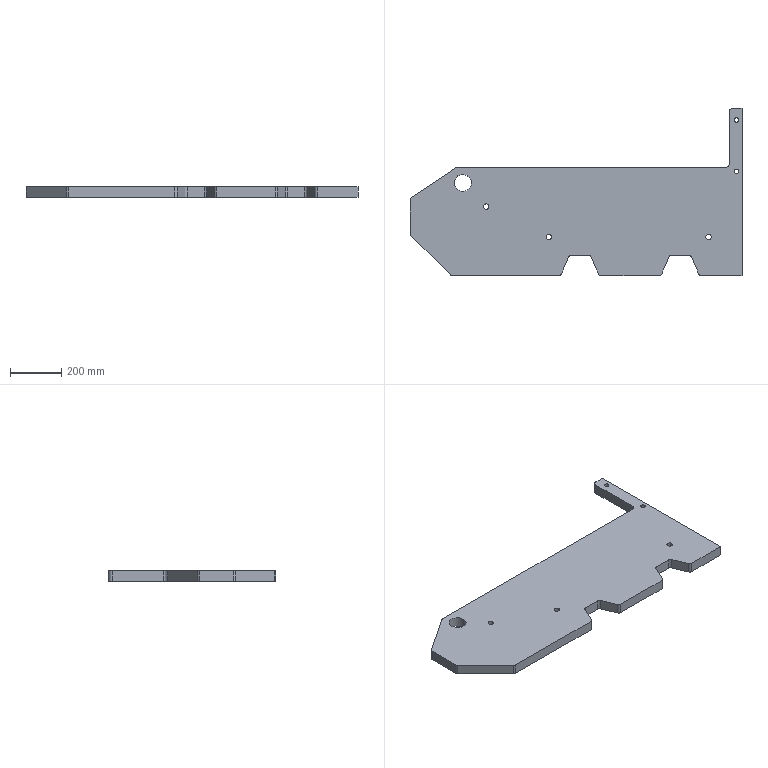Part | SolidWorks | features Fillet 3, Chamfer 2, 3DProfileFeature 1, Extrusion 1, HoleWzd 1, ICE 1 | 1 solid | 44 faces | box 1290 x 650 x 40 mm | volume 20252849 mm3 | cylinder 26 | plane 18 | commonest cylinder face diameters 20 x12 21 x6 18 x4 30 x2 66 x2
STEP:
#1=CARTESIAN_POINT('',(550.5,150.,0.));
#2=VERTEX_POINT('',#1);
#3=CARTESIAN_POINT('',(529.5,150.,0.));
#4=VERTEX_POINT('',#3);
#5=CARTESIAN_POINT('',(540.,150.,0.));
#6=DIRECTION('',(0.,0.,-1.));
#7=DIRECTION('',(-1.,0.,0.));
#8=AXIS2_PLACEMENT_3D('',#5,#6,#7);
#9=CIRCLE('',#8,10.5);
#10=EDGE_CURVE('',#2,#4,#9,.T.);
#11=ORIENTED_EDGE('',*,*,#10,.T.);
#12=CARTESIAN_POINT('',(529.5,150.,40.));
#13=VERTEX_POINT('',#12);
#14=CARTESIAN_POINT('',(529.5,150.,40.));
#15=DIRECTION('',(0.,0.,1.));
#16=VECTOR('',#15,1000.);
#17=LINE('',#14,#16);
#18=EDGE_CURVE('',#4,#13,#17,.T.);
#19=ORIENTED_EDGE('',*,*,#18,.T.);
#20=CARTESIAN_POINT('',(550.5,150.,40.));
#21=VERTEX_POINT('',#20);
#22=CARTESIAN_POINT('',(540.,150.,40.));
#23=DIRECTION('',(0.,0.,1.));
#24=DIRECTION('',(1.,0.,0.));
#25=AXIS2_PLACEMENT_3D('',#22,#23,#24);
#26=CIRCLE('',#25,10.5);
#27=EDGE_CURVE('',#13,#21,#26,.T.);
#28=ORIENTED_EDGE('',*,*,#27,.T.);
#29=CARTESIAN_POINT('',(550.5,150.,40.));
#30=DIRECTION('',(0.,0.,1.));
#31=VECTOR('',#30,1000.);
#32=LINE('',#29,#31);
#33=EDGE_CURVE('',#2,#21,#32,.T.);
#34=ORIENTED_EDGE('',*,*,#33,.F.);
#35=EDGE_LOOP('',(#11,#19,#28,#34));
#36=FACE_OUTER_BOUND('',#35,.T.);
#37=CARTESIAN_POINT('',(540.,150.,40.));
#38=DIRECTION('',(0.,0.,1.));
#39=DIRECTION('',(1.,0.,0.));
#40=AXIS2_PLACEMENT_3D('',#37,#38,#39);
#41=CYLINDRICAL_SURFACE('',#40,10.5);
#42=ADVANCED_FACE('',(#36),#41,.F.);
#43=CARTESIAN_POINT('',(1170.5,150.,0.));
#44=VERTEX_POINT('',#43);
#45=CARTESIAN_POINT('',(1149.5,150.,0.));
#46=VERTEX_POINT('',#45);
#47=CARTESIAN_POINT('',(1160.,150.,0.));
#48=DIRECTION('',(0.,0.,-1.));
#49=DIRECTION('',(-1.,0.,0.));
#50=AXIS2_PLACEMENT_3D('',#47,#48,#49);
#51=CIRCLE('',#50,10.5);
#52=EDGE_CURVE('',#44,#46,#51,.T.);
#53=ORIENTED_EDGE('',*,*,#52,.T.);
#54=CARTESIAN_POINT('',(1149.5,150.,40.));
#55=VERTEX_POINT('',#54);
#56=CARTESIAN_POINT('',(1149.5,150.,40.));
#57=DIRECTION('',(0.,0.,1.));
#58=VECTOR('',#57,1000.);
#59=LINE('',#56,#58);
#60=EDGE_CURVE('',#46,#55,#59,.T.);
#61=ORIENTED_EDGE('',*,*,#60,.T.);
#62=CARTESIAN_POINT('',(1170.5,150.,40.));
#63=VERTEX_POINT('',#62);
#64=CARTESIAN_POINT('',(1160.,150.,40.));
#65=DIRECTION('',(0.,0.,1.));
#66=DIRECTION('',(1.,0.,0.));
#67=AXIS2_PLACEMENT_3D('',#64,#65,#66);
#68=CIRCLE('',#67,10.5);
#69=EDGE_CURVE('',#55,#63,#68,.T.);
#70=ORIENTED_EDGE('',*,*,#69,.T.);
#71=CARTESIAN_POINT('',(1170.5,150.,40.));
#72=DIRECTION('',(0.,0.,1.));
#73=VECTOR('',#72,1000.);
#74=LINE('',#71,#73);
#75=EDGE_CURVE('',#44,#63,#74,.T.);
#76=ORIENTED_EDGE('',*,*,#75,.F.);
#77=EDGE_LOOP('',(#53,#61,#70,#76));
#78=FACE_OUTER_BOUND('',#77,.T.);
#79=CARTESIAN_POINT('',(1160.,150.,40.));
#80=DIRECTION('',(0.,0.,1.));
#81=DIRECTION('',(1.,0.,0.));
#82=AXIS2_PLACEMENT_3D('',#79,#80,#81);
#83=CYLINDRICAL_SURFACE('',#82,10.5);
#84=ADVANCED_FACE('',(#78),#83,.F.);
#85=CARTESIAN_POINT('',(306.435,268.316,0.));
#86=VERTEX_POINT('',#85);
#87=CARTESIAN_POINT('',(285.435,268.316,0.));
#88=VERTEX_POINT('',#87);
#89=CARTESIAN_POINT('',(295.935,268.316,0.));
#90=DIRECTION('',(0.,0.,-1.));
#91=DIRECTION('',(-1.,0.,0.));
#92=AXIS2_PLACEMENT_3D('',#89,#90,#91);
#93=CIRCLE('',#92,10.5);
#94=EDGE_CURVE('',#86,#88,#93,.T.);
#95=ORIENTED_EDGE('',*,*,#94,.T.);
#96=CARTESIAN_POINT('',(285.435,268.316,40.));
#97=VERTEX_POINT('',#96);
#98=CARTESIAN_POINT('',(285.435,268.316,40.));
#99=DIRECTION('',(0.,0.,1.));
#100=VECTOR('',#99,1000.);
#101=LINE('',#98,#100);
#102=EDGE_CURVE('',#88,#97,#101,.T.);
#103=ORIENTED_EDGE('',*,*,#102,.T.);
#104=CARTESIAN_POINT('',(306.435,268.316,40.));
#105=VERTEX_POINT('',#104);
#106=CARTESIAN_POINT('',(295.935,268.316,40.));
#107=DIRECTION('',(0.,0.,1.));
#108=DIRECTION('',(1.,0.,0.));
#109=AXIS2_PLACEMENT_3D('',#106,#107,#108);
#110=CIRCLE('',#109,10.5);
#111=EDGE_CURVE('',#97,#105,#110,.T.);
#112=ORIENTED_EDGE('',*,*,#111,.T.);
#113=CARTESIAN_POINT('',(306.435,268.316,40.));
#114=DIRECTION('',(0.,0.,1.));
#115=VECTOR('',#114,1000.);
#116=LINE('',#113,#115);
#117=EDGE_CURVE('',#86,#105,#116,.T.);
#118=ORIENTED_EDGE('',*,*,#117,.F.);
#119=EDGE_LOOP('',(#95,#103,#112,#118));
#120=FACE_OUTER_BOUND('',#119,.T.);
#121=CARTESIAN_POINT('',(295.935,268.316,40.));
#122=DIRECTION('',(0.,0.,1.));
#123=DIRECTION('',(1.,0.,0.));
#124=AXIS2_PLACEMENT_3D('',#121,#122,#123);
#125=CYLINDRICAL_SURFACE('',#124,10.5);
#126=ADVANCED_FACE('',(#120),#125,.F.);
#127=CARTESIAN_POINT('',(1260.,405.,40.));
#128=VERTEX_POINT('',#127);
#129=CARTESIAN_POINT('',(1278.,405.,40.));
#130=VERTEX_POINT('',#129);
#131=CARTESIAN_POINT('',(1269.,405.,40.));
#132=DIRECTION('',(0.,0.,1.));
#133=DIRECTION('',(1.,0.,0.));
#134=AXIS2_PLACEMENT_3D('',#131,#132,#133);
#135=CIRCLE('',#134,9.);
#136=EDGE_CURVE('',#128,#130,#135,.T.);
#137=ORIENTED_EDGE('',*,*,#136,.T.);
#138=CARTESIAN_POINT('',(1278.,405.,0.));
#139=VERTEX_POINT('',#138);
#140=CARTESIAN_POINT('',(1278.,405.,40.));
#141=DIRECTION('',(0.,0.,-1.));
#142=VECTOR('',#141,1000.);
#143=LINE('',#140,#142);
#144=EDGE_CURVE('',#130,#139,#143,.T.);
#145=ORIENTED_EDGE('',*,*,#144,.T.);
#146=CARTESIAN_POINT('',(1260.,405.,0.));
#147=VERTEX_POINT('',#146);
#148=CARTESIAN_POINT('',(1269.,405.,0.));
#149=DIRECTION('',(0.,0.,1.));
#150=DIRECTION('',(1.,0.,0.));
#151=AXIS2_PLACEMENT_3D('',#148,#149,#150);
#152=CIRCLE('',#151,9.);
#153=EDGE_CURVE('',#147,#139,#152,.T.);
#154=ORIENTED_EDGE('',*,*,#153,.F.);
#155=CARTESIAN_POINT('',(1260.,405.,40.));
#156=DIRECTION('',(0.,0.,-1.));
#157=VECTOR('',#156,1000.);
#158=LINE('',#155,#157);
#159=EDGE_CURVE('',#128,#147,#158,.T.);
#160=ORIENTED_EDGE('',*,*,#159,.F.);
#161=EDGE_LOOP('',(#137,#145,#154,#160));
#162=FACE_OUTER_BOUND('',#161,.T.);
#163=CARTESIAN_POINT('',(1269.,405.,40.));
#164=DIRECTION('',(0.,0.,-1.));
#165=DIRECTION('',(-1.,0.,0.));
#166=AXIS2_PLACEMENT_3D('',#163,#164,#165);
#167=CYLINDRICAL_SURFACE('',#166,9.);
#168=ADVANCED_FACE('',(#162),#167,.F.);
#169=CARTESIAN_POINT('',(1260.,605.,40.));
#170=VERTEX_POINT('',#169);
#171=CARTESIAN_POINT('',(1278.,605.,40.));
#172=VERTEX_POINT('',#171);
#173=CARTESIAN_POINT('',(1269.,605.,40.));
#174=DIRECTION('',(0.,0.,1.));
#175=DIRECTION('',(1.,0.,0.));
#176=AXIS2_PLACEMENT_3D('',#173,#174,#175);
#177=CIRCLE('',#176,9.);
#178=EDGE_CURVE('',#170,#172,#177,.T.);
#179=ORIENTED_EDGE('',*,*,#178,.T.);
#180=CARTESIAN_POINT('',(1278.,605.,0.));
#181=VERTEX_POINT('',#180);
#182=CARTESIAN_POINT('',(1278.,605.,40.));
#183=DIRECTION('',(0.,0.,-1.));
#184=VECTOR('',#183,1000.);
#185=LINE('',#182,#184);
#186=EDGE_CURVE('',#172,#181,#185,.T.);
#187=ORIENTED_EDGE('',*,*,#186,.T.);
#188=CARTESIAN_POINT('',(1260.,605.,0.));
#189=VERTEX_POINT('',#188);
#190=CARTESIAN_POINT('',(1269.,605.,0.));
#191=DIRECTION('',(0.,0.,1.));
#192=DIRECTION('',(1.,0.,0.));
#193=AXIS2_PLACEMENT_3D('',#190,#191,#192);
#194=CIRCLE('',#193,9.);
#195=EDGE_CURVE('',#189,#181,#194,.T.);
#196=ORIENTED_EDGE('',*,*,#195,.F.);
#197=CARTESIAN_POINT('',(1260.,605.,40.));
#198=DIRECTION('',(0.,0.,-1.));
#199=VECTOR('',#198,1000.);
#200=LINE('',#197,#199);
#201=EDGE_CURVE('',#170,#189,#200,.T.);
#202=ORIENTED_EDGE('',*,*,#201,.F.);
#203=EDGE_LOOP('',(#179,#187,#196,#202));
#204=FACE_OUTER_BOUND('',#203,.T.);
#205=CARTESIAN_POINT('',(1269.,605.,40.));
#206=DIRECTION('',(0.,0.,-1.));
#207=DIRECTION('',(-1.,0.,0.));
#208=AXIS2_PLACEMENT_3D('',#205,#206,#207);
#209=CYLINDRICAL_SURFACE('',#208,9.);
#210=ADVANCED_FACE('',(#204),#209,.F.);
#211=CARTESIAN_POINT('',(172.,360.,40.));
#212=VERTEX_POINT('',#211);
#213=CARTESIAN_POINT('',(238.,360.,40.));
#214=VERTEX_POINT('',#213);
#215=CARTESIAN_POINT('',(205.,360.,40.));
#216=DIRECTION('',(0.,0.,1.));
#217=DIRECTION('',(1.,0.,0.));
#218=AXIS2_PLACEMENT_3D('',#215,#216,#217);
#219=CIRCLE('',#218,33.);
#220=EDGE_CURVE('',#212,#214,#219,.T.);
#221=ORIENTED_EDGE('',*,*,#220,.T.);
#222=CARTESIAN_POINT('',(238.,360.,0.));
#223=VERTEX_POINT('',#222);
#224=CARTESIAN_POINT('',(238.,360.,40.));
#225=DIRECTION('',(0.,0.,-1.));
#226=VECTOR('',#225,1000.);
#227=LINE('',#224,#226);
#228=EDGE_CURVE('',#214,#223,#227,.T.);
#229=ORIENTED_EDGE('',*,*,#228,.T.);
#230=CARTESIAN_POINT('',(172.,360.,0.));
#231=VERTEX_POINT('',#230);
#232=CARTESIAN_POINT('',(205.,360.,0.));
#233=DIRECTION('',(0.,0.,1.));
#234=DIRECTION('',(1.,0.,0.));
#235=AXIS2_PLACEMENT_3D('',#232,#233,#234);
#236=CIRCLE('',#235,33.);
#237=EDGE_CURVE('',#231,#223,#236,.T.);
#238=ORIENTED_EDGE('',*,*,#237,.F.);
#239=CARTESIAN_POINT('',(172.,360.,40.));
#240=DIRECTION('',(0.,0.,-1.));
#241=VECTOR('',#240,1000.);
#242=LINE('',#239,#241);
#243=EDGE_CURVE('',#212,#231,#242,.T.);
#244=ORIENTED_EDGE('',*,*,#243,.F.);
#245=EDGE_LOOP('',(#221,#229,#238,#244));
#246=FACE_OUTER_BOUND('',#245,.T.);
#247=CARTESIAN_POINT('',(205.,360.,40.));
#248=DIRECTION('',(0.,0.,-1.));
#249=DIRECTION('',(-1.,0.,0.));
#250=AXIS2_PLACEMENT_3D('',#247,#248,#249);
#251=CYLINDRICAL_SURFACE('',#250,33.);
#252=ADVANCED_FACE('',(#246),#251,.F.);
#253=CARTESIAN_POINT('',(1131.54,0.,40.));
#254=VERTEX_POINT('',#253);
#255=CARTESIAN_POINT('',(1290.,0.,40.));
#256=VERTEX_POINT('',#255);
#257=CARTESIAN_POINT('',(0.,0.,40.));
#258=DIRECTION('',(1.,0.,0.));
#259=VECTOR('',#258,1000.);
#260=LINE('',#257,#259);
#261=EDGE_CURVE('',#254,#256,#260,.T.);
#262=ORIENTED_EDGE('',*,*,#261,.F.);
#263=CARTESIAN_POINT('',(1131.54,0.,0.));
#264=VERTEX_POINT('',#263);
#265=CARTESIAN_POINT('',(1131.54,0.,40.));
#266=DIRECTION('',(0.,0.,-1.));
#267=VECTOR('',#266,1000.);
#268=LINE('',#265,#267);
#269=EDGE_CURVE('',#254,#264,#268,.T.);
#270=ORIENTED_EDGE('',*,*,#269,.T.);
#271=CARTESIAN_POINT('',(1290.,0.,0.));
#272=VERTEX_POINT('',#271);
#273=CARTESIAN_POINT('',(0.,0.,0.));
#274=DIRECTION('',(1.,0.,0.));
#275=VECTOR('',#274,1000.);
#276=LINE('',#273,#275);
#277=EDGE_CURVE('',#264,#272,#276,.T.);
#278=ORIENTED_EDGE('',*,*,#277,.T.);
#279=CARTESIAN_POINT('',(1290.,0.,40.));
#280=DIRECTION('',(0.,0.,-1.));
#281=VECTOR('',#280,1000.);
#282=LINE('',#279,#281);
#283=EDGE_CURVE('',#256,#272,#282,.T.);
#284=ORIENTED_EDGE('',*,*,#283,.F.);
#285=EDGE_LOOP('',(#262,#270,#278,#284));
#286=FACE_OUTER_BOUND('',#285,.T.);
#287=CARTESIAN_POINT('',(0.,0.,40.));
#288=DIRECTION('',(0.,1.,0.));
#289=DIRECTION('',(0.,0.,1.));
#290=AXIS2_PLACEMENT_3D('',#287,#288,#289);
#291=PLANE('',#290);
#292=ADVANCED_FACE('',(#286),#291,.F.);
#293=CARTESIAN_POINT('',(741.54,0.,0.));
#294=VERTEX_POINT('',#293);
#295=CARTESIAN_POINT('',(968.46,0.,0.));
#296=VERTEX_POINT('',#295);
#297=CARTESIAN_POINT('',(0.,0.,0.));
#298=DIRECTION('',(1.,0.,0.));
#299=VECTOR('',#298,1000.);
#300=LINE('',#297,#299);
#301=EDGE_CURVE('',#294,#296,#300,.T.);
#302=ORIENTED_EDGE('',*,*,#301,.T.);
#303=CARTESIAN_POINT('',(968.46,0.,40.));
#304=VERTEX_POINT('',#303);
#305=CARTESIAN_POINT('',(968.46,0.,40.));
#306=DIRECTION('',(0.,0.,1.));
#307=VECTOR('',#306,1000.);
#308=LINE('',#305,#307);
#309=EDGE_CURVE('',#296,#304,#308,.T.);
#310=ORIENTED_EDGE('',*,*,#309,.T.);
#311=CARTESIAN_POINT('',(741.54,0.,40.));
#312=VERTEX_POINT('',#311);
#313=CARTESIAN_POINT('',(0.,0.,40.));
#314=DIRECTION('',(1.,0.,0.));
#315=VECTOR('',#314,1000.);
#316=LINE('',#313,#315);
#317=EDGE_CURVE('',#312,#304,#316,.T.);
#318=ORIENTED_EDGE('',*,*,#317,.F.);
#319=CARTESIAN_POINT('',(741.54,0.,40.));
#320=DIRECTION('',(0.,0.,-1.));
#321=VECTOR('',#320,1000.);
#322=LINE('',#319,#321);
#323=EDGE_CURVE('',#312,#294,#322,.T.);
#324=ORIENTED_EDGE('',*,*,#323,.T.);
#325=EDGE_LOOP('',(#302,#310,#318,#324));
#326=FACE_OUTER_BOUND('',#325,.T.);
#327=CARTESIAN_POINT('',(0.,0.,40.));
#328=DIRECTION('',(0.,1.,0.));
#329=DIRECTION('',(0.,0.,1.));
#330=AXIS2_PLACEMENT_3D('',#327,#328,#329);
#331=PLANE('',#330);
#332=ADVANCED_FACE('',(#326),#331,.F.);
#333=CARTESIAN_POINT('',(540.,150.,40.));
#334=DIRECTION('',(0.,0.,1.));
#335=DIRECTION('',(1.,0.,0.));
#336=AXIS2_PLACEMENT_3D('',#333,#334,#335);
#337=CIRCLE('',#336,10.5);
#338=EDGE_CURVE('',#21,#13,#337,.T.);
#339=ORIENTED_EDGE('',*,*,#338,.F.);
#340=ORIENTED_EDGE('',*,*,#27,.F.);
#341=EDGE_LOOP('',(#339,#340));
#342=FACE_BOUND('',#341,.T.);
#343=CARTESIAN_POINT('',(2.929,157.071,40.));
#344=VERTEX_POINT('',#343);
#345=CARTESIAN_POINT('',(157.071,2.929,40.));
#346=VERTEX_POINT('',#345);
#347=CARTESIAN_POINT('',(160.,0.,40.));
#348=DIRECTION('',(0.7071,-0.7071,0.));
#349=VECTOR('',#348,1000.);
#350=LINE('',#347,#349);
#351=EDGE_CURVE('',#344,#346,#350,.T.);
#352=ORIENTED_EDGE('',*,*,#351,.T.);
#353=CARTESIAN_POINT('',(164.142,0.,40.));
#354=VERTEX_POINT('',#353);
#355=CARTESIAN_POINT('',(164.142,10.,40.));
#356=DIRECTION('',(0.,0.,1.));
#357=DIRECTION('',(-1.,0.,0.));
#358=AXIS2_PLACEMENT_3D('',#355,#356,#357);
#359=CIRCLE('',#358,10.);
#360=EDGE_CURVE('',#346,#354,#359,.T.);
#361=ORIENTED_EDGE('',*,*,#360,.T.);
#362=CARTESIAN_POINT('',(578.46,0.,40.));
#363=VERTEX_POINT('',#362);
#364=CARTESIAN_POINT('',(0.,0.,40.));
#365=DIRECTION('',(1.,0.,0.));
#366=VECTOR('',#365,1000.);
#367=LINE('',#364,#366);
#368=EDGE_CURVE('',#354,#363,#367,.T.);
#369=ORIENTED_EDGE('',*,*,#368,.T.);
#370=CARTESIAN_POINT('',(587.621,5.992,40.));
#371=VERTEX_POINT('',#370);
#372=CARTESIAN_POINT('',(578.46,10.,40.));
#373=DIRECTION('',(0.,0.,1.));
#374=DIRECTION('',(-1.,0.,0.));
#375=AXIS2_PLACEMENT_3D('',#372,#373,#374);
#376=CIRCLE('',#375,10.);
#377=EDGE_CURVE('',#363,#371,#376,.T.);
#378=ORIENTED_EDGE('',*,*,#377,.T.);
#379=CARTESIAN_POINT('',(617.379,74.008,40.));
#380=VERTEX_POINT('',#379);
#381=CARTESIAN_POINT('',(620.,80.,40.));
#382=DIRECTION('',(-0.4008,-0.9162,0.));
#383=VECTOR('',#382,1000.);
#384=LINE('',#381,#383);
#385=EDGE_CURVE('',#380,#371,#384,.T.);
#386=ORIENTED_EDGE('',*,*,#385,.F.);
#387=CARTESIAN_POINT('',(626.54,80.,40.));
#388=VERTEX_POINT('',#387);
#389=CARTESIAN_POINT('',(626.54,70.,40.));
#390=DIRECTION('',(0.,0.,-1.));
#391=DIRECTION('',(-1.,0.,0.));
#392=AXIS2_PLACEMENT_3D('',#389,#390,#391);
#393=CIRCLE('',#392,10.);
#394=EDGE_CURVE('',#380,#388,#393,.T.);
#395=ORIENTED_EDGE('',*,*,#394,.T.);
#396=CARTESIAN_POINT('',(693.46,80.,40.));
#397=VERTEX_POINT('',#396);
#398=CARTESIAN_POINT('',(620.,80.,40.));
#399=DIRECTION('',(-1.,0.,0.));
#400=VECTOR('',#399,1000.);
#401=LINE('',#398,#400);
#402=EDGE_CURVE('',#397,#388,#401,.T.);
#403=ORIENTED_EDGE('',*,*,#402,.F.);
#404=CARTESIAN_POINT('',(702.621,74.008,40.));
#405=VERTEX_POINT('',#404);
#406=CARTESIAN_POINT('',(693.46,70.,40.));
#407=DIRECTION('',(0.,0.,-1.));
#408=DIRECTION('',(-1.,0.,0.));
#409=AXIS2_PLACEMENT_3D('',#406,#407,#408);
#410=CIRCLE('',#409,10.);
#411=EDGE_CURVE('',#397,#405,#410,.T.);
#412=ORIENTED_EDGE('',*,*,#411,.T.);
#413=CARTESIAN_POINT('',(732.379,5.992,40.));
#414=VERTEX_POINT('',#413);
#415=CARTESIAN_POINT('',(700.,80.,40.));
#416=DIRECTION('',(-0.4008,0.9162,0.));
#417=VECTOR('',#416,1000.);
#418=LINE('',#415,#417);
#419=EDGE_CURVE('',#414,#405,#418,.T.);
#420=ORIENTED_EDGE('',*,*,#419,.F.);
#421=CARTESIAN_POINT('',(741.54,10.,40.));
#422=DIRECTION('',(0.,0.,1.));
#423=DIRECTION('',(-1.,0.,0.));
#424=AXIS2_PLACEMENT_3D('',#421,#422,#423);
#425=CIRCLE('',#424,10.);
#426=EDGE_CURVE('',#414,#312,#425,.T.);
#427=ORIENTED_EDGE('',*,*,#426,.T.);
#428=ORIENTED_EDGE('',*,*,#317,.T.);
#429=CARTESIAN_POINT('',(977.621,5.992,40.));
#430=VERTEX_POINT('',#429);
#431=CARTESIAN_POINT('',(968.46,10.,40.));
#432=DIRECTION('',(0.,0.,1.));
#433=DIRECTION('',(-1.,0.,0.));
#434=AXIS2_PLACEMENT_3D('',#431,#432,#433);
#435=CIRCLE('',#434,10.);
#436=EDGE_CURVE('',#304,#430,#435,.T.);
#437=ORIENTED_EDGE('',*,*,#436,.T.);
#438=CARTESIAN_POINT('',(1007.379,74.008,40.));
#439=VERTEX_POINT('',#438);
#440=CARTESIAN_POINT('',(1010.,80.,40.));
#441=DIRECTION('',(-0.4008,-0.9162,0.));
#442=VECTOR('',#441,1000.);
#443=LINE('',#440,#442);
#444=EDGE_CURVE('',#439,#430,#443,.T.);
#445=ORIENTED_EDGE('',*,*,#444,.F.);
#446=CARTESIAN_POINT('',(1016.54,80.,40.));
#447=VERTEX_POINT('',#446);
#448=CARTESIAN_POINT('',(1016.54,70.,40.));
#449=DIRECTION('',(0.,0.,-1.));
#450=DIRECTION('',(-1.,0.,0.));
#451=AXIS2_PLACEMENT_3D('',#448,#449,#450);
#452=CIRCLE('',#451,10.);
#453=EDGE_CURVE('',#439,#447,#452,.T.);
#454=ORIENTED_EDGE('',*,*,#453,.T.);
#455=CARTESIAN_POINT('',(1083.46,80.,40.));
#456=VERTEX_POINT('',#455);
#457=CARTESIAN_POINT('',(1010.,80.,40.));
#458=DIRECTION('',(-1.,0.,0.));
#459=VECTOR('',#458,1000.);
#460=LINE('',#457,#459);
#461=EDGE_CURVE('',#456,#447,#460,.T.);
#462=ORIENTED_EDGE('',*,*,#461,.F.);
#463=CARTESIAN_POINT('',(1092.621,74.008,40.));
#464=VERTEX_POINT('',#463);
#465=CARTESIAN_POINT('',(1083.46,70.,40.));
#466=DIRECTION('',(0.,0.,-1.));
#467=DIRECTION('',(-1.,0.,0.));
#468=AXIS2_PLACEMENT_3D('',#465,#466,#467);
#469=CIRCLE('',#468,10.);
#470=EDGE_CURVE('',#456,#464,#469,.T.);
#471=ORIENTED_EDGE('',*,*,#470,.T.);
#472=CARTESIAN_POINT('',(1122.379,5.992,40.));
#473=VERTEX_POINT('',#472);
#474=CARTESIAN_POINT('',(1090.,80.,40.));
#475=DIRECTION('',(-0.4008,0.9162,0.));
#476=VECTOR('',#475,1000.);
#477=LINE('',#474,#476);
#478=EDGE_CURVE('',#473,#464,#477,.T.);
#479=ORIENTED_EDGE('',*,*,#478,.F.);
#480=CARTESIAN_POINT('',(1131.54,10.,40.));
#481=DIRECTION('',(0.,0.,1.));
#482=DIRECTION('',(-1.,0.,0.));
#483=AXIS2_PLACEMENT_3D('',#480,#481,#482);
#484=CIRCLE('',#483,10.);
#485=EDGE_CURVE('',#473,#254,#484,.T.);
#486=ORIENTED_EDGE('',*,*,#485,.T.);
#487=ORIENTED_EDGE('',*,*,#261,.T.);
#488=CARTESIAN_POINT('',(1290.,650.,40.));
#489=VERTEX_POINT('',#488);
#490=CARTESIAN_POINT('',(1290.,0.,40.));
#491=DIRECTION('',(0.,1.,0.));
#492=VECTOR('',#491,1000.);
#493=LINE('',#490,#492);
#494=EDGE_CURVE('',#256,#489,#493,.T.);
#495=ORIENTED_EDGE('',*,*,#494,.T.);
#496=CARTESIAN_POINT('',(1255.,650.,40.));
#497=VERTEX_POINT('',#496);
#498=CARTESIAN_POINT('',(1240.,650.,40.));
#499=DIRECTION('',(-1.,0.,0.));
#500=VECTOR('',#499,1000.);
#501=LINE('',#498,#500);
#502=EDGE_CURVE('',#489,#497,#501,.T.);
#503=ORIENTED_EDGE('',*,*,#502,.T.);
#504=CARTESIAN_POINT('',(1240.,635.,40.));
#505=VERTEX_POINT('',#504);
#506=CARTESIAN_POINT('',(1255.,635.,40.));
#507=DIRECTION('',(0.,0.,1.));
#508=DIRECTION('',(-1.,0.,0.));
#509=AXIS2_PLACEMENT_3D('',#506,#507,#508);
#510=CIRCLE('',#509,15.);
#511=EDGE_CURVE('',#497,#505,#510,.T.);
#512=ORIENTED_EDGE('',*,*,#511,.T.);
#513=CARTESIAN_POINT('',(1240.,435.,40.));
#514=VERTEX_POINT('',#513);
#515=CARTESIAN_POINT('',(1240.,420.,40.));
#516=DIRECTION('',(0.,-1.,0.));
#517=VECTOR('',#516,1000.);
#518=LINE('',#515,#517);
#519=EDGE_CURVE('',#505,#514,#518,.T.);
#520=ORIENTED_EDGE('',*,*,#519,.T.);
#521=CARTESIAN_POINT('',(1225.,420.,40.));
#522=VERTEX_POINT('',#521);
#523=CARTESIAN_POINT('',(1225.,435.,40.));
#524=DIRECTION('',(0.,0.,-1.));
#525=DIRECTION('',(-1.,0.,0.));
#526=AXIS2_PLACEMENT_3D('',#523,#524,#525);
#527=CIRCLE('',#526,15.);
#528=EDGE_CURVE('',#514,#522,#527,.T.);
#529=ORIENTED_EDGE('',*,*,#528,.T.);
#530=CARTESIAN_POINT('',(183.028,420.,40.));
#531=VERTEX_POINT('',#530);
#532=CARTESIAN_POINT('',(0.,420.,40.));
#533=DIRECTION('',(-1.,0.,0.));
#534=VECTOR('',#533,1000.);
#535=LINE('',#532,#534);
#536=EDGE_CURVE('',#522,#531,#535,.T.);
#537=ORIENTED_EDGE('',*,*,#536,.T.);
#538=CARTESIAN_POINT('',(177.481,418.321,40.));
#539=VERTEX_POINT('',#538);
#540=CARTESIAN_POINT('',(183.028,410.,40.));
#541=DIRECTION('',(0.,0.,1.));
#542=DIRECTION('',(-1.,0.,0.));
#543=AXIS2_PLACEMENT_3D('',#540,#541,#542);
#544=CIRCLE('',#543,10.);
#545=EDGE_CURVE('',#531,#539,#544,.T.);
#546=ORIENTED_EDGE('',*,*,#545,.T.);
#547=CARTESIAN_POINT('',(4.453,302.969,40.));
#548=VERTEX_POINT('',#547);
#549=CARTESIAN_POINT('',(0.,300.,40.));
#550=DIRECTION('',(-0.8321,-0.5547,0.));
#551=VECTOR('',#550,1000.);
#552=LINE('',#549,#551);
#553=EDGE_CURVE('',#539,#548,#552,.T.);
#554=ORIENTED_EDGE('',*,*,#553,.T.);
#555=CARTESIAN_POINT('',(0.,294.648,40.));
#556=VERTEX_POINT('',#555);
#557=CARTESIAN_POINT('',(10.,294.648,40.));
#558=DIRECTION('',(0.,0.,1.));
#559=DIRECTION('',(-1.,0.,0.));
#560=AXIS2_PLACEMENT_3D('',#557,#558,#559);
#561=CIRCLE('',#560,10.);
#562=EDGE_CURVE('',#548,#556,#561,.T.);
#563=ORIENTED_EDGE('',*,*,#562,.T.);
#564=CARTESIAN_POINT('',(0.,164.142,40.));
#565=VERTEX_POINT('',#564);
#566=CARTESIAN_POINT('',(0.,0.,40.));
#567=DIRECTION('',(0.,-1.,0.));
#568=VECTOR('',#567,1000.);
#569=LINE('',#566,#568);
#570=EDGE_CURVE('',#556,#565,#569,.T.);
#571=ORIENTED_EDGE('',*,*,#570,.T.);
#572=CARTESIAN_POINT('',(10.,164.142,40.));
#573=DIRECTION('',(0.,0.,1.));
#574=DIRECTION('',(-1.,0.,0.));
#575=AXIS2_PLACEMENT_3D('',#572,#573,#574);
#576=CIRCLE('',#575,10.);
#577=EDGE_CURVE('',#565,#344,#576,.T.);
#578=ORIENTED_EDGE('',*,*,#577,.T.);
#579=EDGE_LOOP('',(#352,#361,#369,#378,#386,#395,#403,#412,#420,#427,#428,#437,#445,#454,#462,#471,#479,#486,#487,#495,#503,#512,#520,#529,#537,#546,#554,#563,#571,#578));
#580=FACE_OUTER_BOUND('',#579,.T.);
#581=ORIENTED_EDGE('',*,*,#220,.F.);
#582=CARTESIAN_POINT('',(205.,360.,40.));
#583=DIRECTION('',(0.,0.,1.));
#584=DIRECTION('',(1.,0.,0.));
#585=AXIS2_PLACEMENT_3D('',#582,#583,#584);
#586=CIRCLE('',#585,33.);
#587=EDGE_CURVE('',#214,#212,#586,.T.);
#588=ORIENTED_EDGE('',*,*,#587,.F.);
#589=EDGE_LOOP('',(#581,#588));
#590=FACE_BOUND('',#589,.T.);
#591=ORIENTED_EDGE('',*,*,#178,.F.);
#592=CARTESIAN_POINT('',(1269.,605.,40.));
#593=DIRECTION('',(0.,0.,1.));
#594=DIRECTION('',(1.,0.,0.));
#595=AXIS2_PLACEMENT_3D('',#592,#593,#594);
#596=CIRCLE('',#595,9.);
#597=EDGE_CURVE('',#172,#170,#596,.T.);
#598=ORIENTED_EDGE('',*,*,#597,.F.);
#599=EDGE_LOOP('',(#591,#598));
#600=FACE_BOUND('',#599,.T.);
#601=ORIENTED_EDGE('',*,*,#136,.F.);
#602=CARTESIAN_POINT('',(1269.,405.,40.));
#603=DIRECTION('',(0.,0.,1.));
#604=DIRECTION('',(1.,0.,0.));
#605=AXIS2_PLACEMENT_3D('',#602,#603,#604);
#606=CIRCLE('',#605,9.);
#607=EDGE_CURVE('',#130,#128,#606,.T.);
#608=ORIENTED_EDGE('',*,*,#607,.F.);
#609=EDGE_LOOP('',(#601,#608));
#610=FACE_BOUND('',#609,.T.);
#611=CARTESIAN_POINT('',(295.935,268.316,40.));
#612=DIRECTION('',(0.,0.,1.));
#613=DIRECTION('',(1.,0.,0.));
#614=AXIS2_PLACEMENT_3D('',#611,#612,#613);
#615=CIRCLE('',#614,10.5);
#616=EDGE_CURVE('',#105,#97,#615,.T.);
#617=ORIENTED_EDGE('',*,*,#616,.F.);
#618=ORIENTED_EDGE('',*,*,#111,.F.);
#619=EDGE_LOOP('',(#617,#618));
#620=FACE_BOUND('',#619,.T.);
#621=CARTESIAN_POINT('',(1160.,150.,40.));
#622=DIRECTION('',(0.,0.,1.));
#623=DIRECTION('',(1.,0.,0.));
#624=AXIS2_PLACEMENT_3D('',#621,#622,#623);
#625=CIRCLE('',#624,10.5);
#626=EDGE_CURVE('',#63,#55,#625,.T.);
#627=ORIENTED_EDGE('',*,*,#626,.F.);
#628=ORIENTED_EDGE('',*,*,#69,.F.);
#629=EDGE_LOOP('',(#627,#628));
#630=FACE_BOUND('',#629,.T.);
#631=CARTESIAN_POINT('',(0.,0.,40.));
#632=DIRECTION('',(0.,0.,-1.));
#633=DIRECTION('',(-1.,0.,0.));
#634=AXIS2_PLACEMENT_3D('',#631,#632,#633);
#635=PLANE('',#634);
#636=ADVANCED_FACE('',(#342,#580,#590,#600,#610,#620,#630),#635,.F.);
#637=CARTESIAN_POINT('',(164.142,0.,0.));
#638=VERTEX_POINT('',#637);
#639=CARTESIAN_POINT('',(578.46,0.,0.));
#640=VERTEX_POINT('',#639);
#641=CARTESIAN_POINT('',(0.,0.,0.));
#642=DIRECTION('',(1.,0.,0.));
#643=VECTOR('',#642,1000.);
#644=LINE('',#641,#643);
#645=EDGE_CURVE('',#638,#640,#644,.T.);
#646=ORIENTED_EDGE('',*,*,#645,.F.);
#647=CARTESIAN_POINT('',(157.071,2.929,0.));
#648=VERTEX_POINT('',#647);
#649=CARTESIAN_POINT('',(164.142,10.,0.));
#650=DIRECTION('',(0.,0.,-1.));
#651=DIRECTION('',(-1.,0.,0.));
#652=AXIS2_PLACEMENT_3D('',#649,#650,#651);
#653=CIRCLE('',#652,10.);
#654=EDGE_CURVE('',#638,#648,#653,.T.);
#655=ORIENTED_EDGE('',*,*,#654,.T.);
#656=CARTESIAN_POINT('',(2.929,157.071,0.));
#657=VERTEX_POINT('',#656);
#658=CARTESIAN_POINT('',(80.,80.,0.));
#659=DIRECTION('',(-0.7071,0.7071,0.));
#660=VECTOR('',#659,1000.);
#661=LINE('',#658,#660);
#662=EDGE_CURVE('',#648,#657,#661,.T.);
#663=ORIENTED_EDGE('',*,*,#662,.T.);
#664=CARTESIAN_POINT('',(0.,164.142,0.));
#665=VERTEX_POINT('',#664);
#666=CARTESIAN_POINT('',(10.,164.142,0.));
#667=DIRECTION('',(0.,0.,-1.));
#668=DIRECTION('',(-1.,0.,0.));
#669=AXIS2_PLACEMENT_3D('',#666,#667,#668);
#670=CIRCLE('',#669,10.);
#671=EDGE_CURVE('',#657,#665,#670,.T.);
#672=ORIENTED_EDGE('',*,*,#671,.T.);
#673=CARTESIAN_POINT('',(0.,294.648,0.));
#674=VERTEX_POINT('',#673);
#675=CARTESIAN_POINT('',(0.,0.,0.));
#676=DIRECTION('',(0.,-1.,0.));
#677=VECTOR('',#676,1000.);
#678=LINE('',#675,#677);
#679=EDGE_CURVE('',#674,#665,#678,.T.);
#680=ORIENTED_EDGE('',*,*,#679,.F.);
#681=CARTESIAN_POINT('',(4.453,302.969,0.));
#682=VERTEX_POINT('',#681);
#683=CARTESIAN_POINT('',(10.,294.648,0.));
#684=DIRECTION('',(0.,0.,-1.));
#685=DIRECTION('',(-1.,0.,0.));
#686=AXIS2_PLACEMENT_3D('',#683,#684,#685);
#687=CIRCLE('',#686,10.);
#688=EDGE_CURVE('',#674,#682,#687,.T.);
#689=ORIENTED_EDGE('',*,*,#688,.T.);
#690=CARTESIAN_POINT('',(177.481,418.321,0.));
#691=VERTEX_POINT('',#690);
#692=CARTESIAN_POINT('',(-138.462,207.692,0.));
#693=DIRECTION('',(0.8321,0.5547,0.));
#694=VECTOR('',#693,1000.);
#695=LINE('',#692,#694);
#696=EDGE_CURVE('',#682,#691,#695,.T.);
#697=ORIENTED_EDGE('',*,*,#696,.T.);
#698=CARTESIAN_POINT('',(183.028,420.,0.));
#699=VERTEX_POINT('',#698);
#700=CARTESIAN_POINT('',(183.028,410.,0.));
#701=DIRECTION('',(0.,0.,-1.));
#702=DIRECTION('',(-1.,0.,0.));
#703=AXIS2_PLACEMENT_3D('',#700,#701,#702);
#704=CIRCLE('',#703,10.);
#705=EDGE_CURVE('',#691,#699,#704,.T.);
#706=ORIENTED_EDGE('',*,*,#705,.T.);
#707=CARTESIAN_POINT('',(1225.,420.,0.));
#708=VERTEX_POINT('',#707);
#709=CARTESIAN_POINT('',(0.,420.,0.));
#710=DIRECTION('',(-1.,0.,0.));
#711=VECTOR('',#710,1000.);
#712=LINE('',#709,#711);
#713=EDGE_CURVE('',#708,#699,#712,.T.);
#714=ORIENTED_EDGE('',*,*,#713,.F.);
#715=CARTESIAN_POINT('',(1240.,435.,0.));
#716=VERTEX_POINT('',#715);
#717=CARTESIAN_POINT('',(1225.,435.,0.));
#718=DIRECTION('',(0.,0.,1.));
#719=DIRECTION('',(-1.,0.,0.));
#720=AXIS2_PLACEMENT_3D('',#717,#718,#719);
#721=CIRCLE('',#720,15.);
#722=EDGE_CURVE('',#708,#716,#721,.T.);
#723=ORIENTED_EDGE('',*,*,#722,.T.);
#724=CARTESIAN_POINT('',(1240.,635.,0.));
#725=VERTEX_POINT('',#724);
#726=CARTESIAN_POINT('',(1240.,420.,0.));
#727=DIRECTION('',(0.,-1.,0.));
#728=VECTOR('',#727,1000.);
#729=LINE('',#726,#728);
#730=EDGE_CURVE('',#725,#716,#729,.T.);
#731=ORIENTED_EDGE('',*,*,#730,.F.);
#732=CARTESIAN_POINT('',(1255.,650.,0.));
#733=VERTEX_POINT('',#732);
#734=CARTESIAN_POINT('',(1255.,635.,0.));
#735=DIRECTION('',(0.,0.,-1.));
#736=DIRECTION('',(-1.,0.,0.));
#737=AXIS2_PLACEMENT_3D('',#734,#735,#736);
#738=CIRCLE('',#737,15.);
#739=EDGE_CURVE('',#725,#733,#738,.T.);
#740=ORIENTED_EDGE('',*,*,#739,.T.);
#741=CARTESIAN_POINT('',(1290.,650.,0.));
#742=VERTEX_POINT('',#741);
#743=CARTESIAN_POINT('',(1240.,650.,0.));
#744=DIRECTION('',(-1.,0.,0.));
#745=VECTOR('',#744,1000.);
#746=LINE('',#743,#745);
#747=EDGE_CURVE('',#742,#733,#746,.T.);
#748=ORIENTED_EDGE('',*,*,#747,.F.);
#749=CARTESIAN_POINT('',(1290.,0.,0.));
#750=DIRECTION('',(0.,1.,0.));
#751=VECTOR('',#750,1000.);
#752=LINE('',#749,#751);
#753=EDGE_CURVE('',#272,#742,#752,.T.);
#754=ORIENTED_EDGE('',*,*,#753,.F.);
#755=ORIENTED_EDGE('',*,*,#277,.F.);
#756=CARTESIAN_POINT('',(1122.379,5.992,0.));
#757=VERTEX_POINT('',#756);
#758=CARTESIAN_POINT('',(1131.54,10.,0.));
#759=DIRECTION('',(0.,0.,-1.));
#760=DIRECTION('',(-1.,0.,0.));
#761=AXIS2_PLACEMENT_3D('',#758,#759,#760);
#762=CIRCLE('',#761,10.);
#763=EDGE_CURVE('',#264,#757,#762,.T.);
#764=ORIENTED_EDGE('',*,*,#763,.T.);
#765=CARTESIAN_POINT('',(1092.621,74.008,0.));
#766=VERTEX_POINT('',#765);
#767=CARTESIAN_POINT('',(1090.,80.,0.));
#768=DIRECTION('',(-0.4008,0.9162,0.));
#769=VECTOR('',#768,1000.);
#770=LINE('',#767,#769);
#771=EDGE_CURVE('',#757,#766,#770,.T.);
#772=ORIENTED_EDGE('',*,*,#771,.T.);
#773=CARTESIAN_POINT('',(1083.46,80.,0.));
#774=VERTEX_POINT('',#773);
#775=CARTESIAN_POINT('',(1083.46,70.,0.));
#776=DIRECTION('',(0.,0.,1.));
#777=DIRECTION('',(-1.,0.,0.));
#778=AXIS2_PLACEMENT_3D('',#775,#776,#777);
#779=CIRCLE('',#778,10.);
#780=EDGE_CURVE('',#766,#774,#779,.T.);
#781=ORIENTED_EDGE('',*,*,#780,.T.);
#782=CARTESIAN_POINT('',(1016.54,80.,0.));
#783=VERTEX_POINT('',#782);
#784=CARTESIAN_POINT('',(1010.,80.,0.));
#785=DIRECTION('',(-1.,0.,0.));
#786=VECTOR('',#785,1000.);
#787=LINE('',#784,#786);
#788=EDGE_CURVE('',#774,#783,#787,.T.);
#789=ORIENTED_EDGE('',*,*,#788,.T.);
#790=CARTESIAN_POINT('',(1007.379,74.008,0.));
#791=VERTEX_POINT('',#790);
#792=CARTESIAN_POINT('',(1016.54,70.,0.));
#793=DIRECTION('',(0.,0.,1.));
#794=DIRECTION('',(-1.,0.,0.));
#795=AXIS2_PLACEMENT_3D('',#792,#793,#794);
#796=CIRCLE('',#795,10.);
#797=EDGE_CURVE('',#783,#791,#796,.T.);
#798=ORIENTED_EDGE('',*,*,#797,.T.);
#799=CARTESIAN_POINT('',(977.621,5.992,0.));
#800=VERTEX_POINT('',#799);
#801=CARTESIAN_POINT('',(1010.,80.,0.));
#802=DIRECTION('',(-0.4008,-0.9162,0.));
#803=VECTOR('',#802,1000.);
#804=LINE('',#801,#803);
#805=EDGE_CURVE('',#791,#800,#804,.T.);
#806=ORIENTED_EDGE('',*,*,#805,.T.);
#807=CARTESIAN_POINT('',(968.46,10.,0.));
#808=DIRECTION('',(0.,0.,-1.));
#809=DIRECTION('',(-1.,0.,0.));
#810=AXIS2_PLACEMENT_3D('',#807,#808,#809);
#811=CIRCLE('',#810,10.);
#812=EDGE_CURVE('',#800,#296,#811,.T.);
#813=ORIENTED_EDGE('',*,*,#812,.T.);
#814=ORIENTED_EDGE('',*,*,#301,.F.);
#815=CARTESIAN_POINT('',(732.379,5.992,0.));
#816=VERTEX_POINT('',#815);
#817=CARTESIAN_POINT('',(741.54,10.,0.));
#818=DIRECTION('',(0.,0.,-1.));
#819=DIRECTION('',(-1.,0.,0.));
#820=AXIS2_PLACEMENT_3D('',#817,#818,#819);
#821=CIRCLE('',#820,10.);
#822=EDGE_CURVE('',#294,#816,#821,.T.);
#823=ORIENTED_EDGE('',*,*,#822,.T.);
#824=CARTESIAN_POINT('',(702.621,74.008,0.));
#825=VERTEX_POINT('',#824);
#826=CARTESIAN_POINT('',(700.,80.,0.));
#827=DIRECTION('',(-0.4008,0.9162,0.));
#828=VECTOR('',#827,1000.);
#829=LINE('',#826,#828);
#830=EDGE_CURVE('',#816,#825,#829,.T.);
#831=ORIENTED_EDGE('',*,*,#830,.T.);
#832=CARTESIAN_POINT('',(693.46,80.,0.));
#833=VERTEX_POINT('',#832);
#834=CARTESIAN_POINT('',(693.46,70.,0.));
#835=DIRECTION('',(0.,0.,1.));
#836=DIRECTION('',(-1.,0.,0.));
#837=AXIS2_PLACEMENT_3D('',#834,#835,#836);
#838=CIRCLE('',#837,10.);
#839=EDGE_CURVE('',#825,#833,#838,.T.);
#840=ORIENTED_EDGE('',*,*,#839,.T.);
#841=CARTESIAN_POINT('',(626.54,80.,0.));
#842=VERTEX_POINT('',#841);
#843=CARTESIAN_POINT('',(620.,80.,0.));
#844=DIRECTION('',(-1.,0.,0.));
#845=VECTOR('',#844,1000.);
#846=LINE('',#843,#845);
#847=EDGE_CURVE('',#833,#842,#846,.T.);
#848=ORIENTED_EDGE('',*,*,#847,.T.);
#849=CARTESIAN_POINT('',(617.379,74.008,0.));
#850=VERTEX_POINT('',#849);
#851=CARTESIAN_POINT('',(626.54,70.,0.));
#852=DIRECTION('',(0.,0.,1.));
#853=DIRECTION('',(-1.,0.,0.));
#854=AXIS2_PLACEMENT_3D('',#851,#852,#853);
#855=CIRCLE('',#854,10.);
#856=EDGE_CURVE('',#842,#850,#855,.T.);
#857=ORIENTED_EDGE('',*,*,#856,.T.);
#858=CARTESIAN_POINT('',(587.621,5.992,0.));
#859=VERTEX_POINT('',#858);
#860=CARTESIAN_POINT('',(620.,80.,0.));
#861=DIRECTION('',(-0.4008,-0.9162,0.));
#862=VECTOR('',#861,1000.);
#863=LINE('',#860,#862);
#864=EDGE_CURVE('',#850,#859,#863,.T.);
#865=ORIENTED_EDGE('',*,*,#864,.T.);
#866=CARTESIAN_POINT('',(578.46,10.,0.));
#867=DIRECTION('',(0.,0.,-1.));
#868=DIRECTION('',(-1.,0.,0.));
#869=AXIS2_PLACEMENT_3D('',#866,#867,#868);
#870=CIRCLE('',#869,10.);
#871=EDGE_CURVE('',#859,#640,#870,.T.);
#872=ORIENTED_EDGE('',*,*,#871,.T.);
#873=EDGE_LOOP('',(#646,#655,#663,#672,#680,#689,#697,#706,#714,#723,#731,#740,#748,#754,#755,#764,#772,#781,#789,#798,#806,#813,#814,#823,#831,#840,#848,#857,#865,#872));
#874=FACE_OUTER_BOUND('',#873,.T.);
#875=ORIENTED_EDGE('',*,*,#10,.F.);
#876=CARTESIAN_POINT('',(540.,150.,0.));
#877=DIRECTION('',(0.,0.,-1.));
#878=DIRECTION('',(-1.,0.,0.));
#879=AXIS2_PLACEMENT_3D('',#876,#877,#878);
#880=CIRCLE('',#879,10.5);
#881=EDGE_CURVE('',#4,#2,#880,.T.);
#882=ORIENTED_EDGE('',*,*,#881,.F.);
#883=EDGE_LOOP('',(#875,#882));
#884=FACE_BOUND('',#883,.T.);
#885=ORIENTED_EDGE('',*,*,#52,.F.);
#886=CARTESIAN_POINT('',(1160.,150.,0.));
#887=DIRECTION('',(0.,0.,-1.));
#888=DIRECTION('',(-1.,0.,0.));
#889=AXIS2_PLACEMENT_3D('',#886,#887,#888);
#890=CIRCLE('',#889,10.5);
#891=EDGE_CURVE('',#46,#44,#890,.T.);
#892=ORIENTED_EDGE('',*,*,#891,.F.);
#893=EDGE_LOOP('',(#885,#892));
#894=FACE_BOUND('',#893,.T.);
#895=ORIENTED_EDGE('',*,*,#94,.F.);
#896=CARTESIAN_POINT('',(295.935,268.316,0.));
#897=DIRECTION('',(0.,0.,-1.));
#898=DIRECTION('',(-1.,0.,0.));
#899=AXIS2_PLACEMENT_3D('',#896,#897,#898);
#900=CIRCLE('',#899,10.5);
#901=EDGE_CURVE('',#88,#86,#900,.T.);
#902=ORIENTED_EDGE('',*,*,#901,.F.);
#903=EDGE_LOOP('',(#895,#902));
#904=FACE_BOUND('',#903,.T.);
#905=ORIENTED_EDGE('',*,*,#195,.T.);
#906=CARTESIAN_POINT('',(1269.,605.,0.));
#907=DIRECTION('',(0.,0.,1.));
#908=DIRECTION('',(1.,0.,0.));
#909=AXIS2_PLACEMENT_3D('',#906,#907,#908);
#910=CIRCLE('',#909,9.);
#911=EDGE_CURVE('',#181,#189,#910,.T.);
#912=ORIENTED_EDGE('',*,*,#911,.T.);
#913=EDGE_LOOP('',(#905,#912));
#914=FACE_BOUND('',#913,.T.);
#915=ORIENTED_EDGE('',*,*,#237,.T.);
#916=CARTESIAN_POINT('',(205.,360.,0.));
#917=DIRECTION('',(0.,0.,1.));
#918=DIRECTION('',(1.,0.,0.));
#919=AXIS2_PLACEMENT_3D('',#916,#917,#918);
#920=CIRCLE('',#919,33.);
#921=EDGE_CURVE('',#223,#231,#920,.T.);
#922=ORIENTED_EDGE('',*,*,#921,.T.);
#923=EDGE_LOOP('',(#915,#922));
#924=FACE_BOUND('',#923,.T.);
#925=ORIENTED_EDGE('',*,*,#153,.T.);
#926=CARTESIAN_POINT('',(1269.,405.,0.));
#927=DIRECTION('',(0.,0.,1.));
#928=DIRECTION('',(1.,0.,0.));
#929=AXIS2_PLACEMENT_3D('',#926,#927,#928);
#930=CIRCLE('',#929,9.);
#931=EDGE_CURVE('',#139,#147,#930,.T.);
#932=ORIENTED_EDGE('',*,*,#931,.T.);
#933=EDGE_LOOP('',(#925,#932));
#934=FACE_BOUND('',#933,.T.);
#935=CARTESIAN_POINT('',(0.,0.,0.));
#936=DIRECTION('',(0.,0.,-1.));
#937=DIRECTION('',(-1.,0.,0.));
#938=AXIS2_PLACEMENT_3D('',#935,#936,#937);
#939=PLANE('',#938);
#940=ADVANCED_FACE('',(#874,#884,#894,#904,#914,#924,#934),#939,.T.);
#941=ORIENTED_EDGE('',*,*,#679,.T.);
#942=CARTESIAN_POINT('',(0.,164.142,40.));
#943=DIRECTION('',(0.,0.,1.));
#944=VECTOR('',#943,1000.);
#945=LINE('',#942,#944);
#946=EDGE_CURVE('',#665,#565,#945,.T.);
#947=ORIENTED_EDGE('',*,*,#946,.T.);
#948=ORIENTED_EDGE('',*,*,#570,.F.);
#949=CARTESIAN_POINT('',(0.,294.648,0.));
#950=DIRECTION('',(0.,0.,-1.));
#951=VECTOR('',#950,1000.);
#952=LINE('',#949,#951);
#953=EDGE_CURVE('',#556,#674,#952,.T.);
#954=ORIENTED_EDGE('',*,*,#953,.T.);
#955=EDGE_LOOP('',(#941,#947,#948,#954));
#956=FACE_OUTER_BOUND('',#955,.T.);
#957=CARTESIAN_POINT('',(0.,0.,40.));
#958=DIRECTION('',(1.,0.,0.));
#959=DIRECTION('',(0.,0.,-1.));
#960=AXIS2_PLACEMENT_3D('',#957,#958,#959);
#961=PLANE('',#960);
#962=ADVANCED_FACE('',(#956),#961,.F.);
#963=ORIENTED_EDGE('',*,*,#368,.F.);
#964=CARTESIAN_POINT('',(164.142,0.,0.));
#965=DIRECTION('',(0.,0.,-1.));
#966=VECTOR('',#965,1000.);
#967=LINE('',#964,#966);
#968=EDGE_CURVE('',#354,#638,#967,.T.);
#969=ORIENTED_EDGE('',*,*,#968,.T.);
#970=ORIENTED_EDGE('',*,*,#645,.T.);
#971=CARTESIAN_POINT('',(578.46,0.,40.));
#972=DIRECTION('',(0.,0.,1.));
#973=VECTOR('',#972,1000.);
#974=LINE('',#971,#973);
#975=EDGE_CURVE('',#640,#363,#974,.T.);
#976=ORIENTED_EDGE('',*,*,#975,.T.);
#977=EDGE_LOOP('',(#963,#969,#970,#976));
#978=FACE_OUTER_BOUND('',#977,.T.);
#979=CARTESIAN_POINT('',(0.,0.,40.));
#980=DIRECTION('',(0.,1.,0.));
#981=DIRECTION('',(0.,0.,1.));
#982=AXIS2_PLACEMENT_3D('',#979,#980,#981);
#983=PLANE('',#982);
#984=ADVANCED_FACE('',(#978),#983,.F.);
#985=ORIENTED_EDGE('',*,*,#753,.T.);
#986=CARTESIAN_POINT('',(1290.,650.,40.));
#987=DIRECTION('',(0.,0.,-1.));
#988=VECTOR('',#987,1000.);
#989=LINE('',#986,#988);
#990=EDGE_CURVE('',#489,#742,#989,.T.);
#991=ORIENTED_EDGE('',*,*,#990,.F.);
#992=ORIENTED_EDGE('',*,*,#494,.F.);
#993=ORIENTED_EDGE('',*,*,#283,.T.);
#994=EDGE_LOOP('',(#985,#991,#992,#993));
#995=FACE_OUTER_BOUND('',#994,.T.);
#996=CARTESIAN_POINT('',(1290.,0.,40.));
#997=DIRECTION('',(-1.,0.,0.));
#998=DIRECTION('',(0.,0.,1.));
#999=AXIS2_PLACEMENT_3D('',#996,#997,#998);
#1000=PLANE('',#999);
#1001=ADVANCED_FACE('',(#995),#1000,.F.);
#1002=ORIENTED_EDGE('',*,*,#747,.T.);
#1003=CARTESIAN_POINT('',(1255.,650.,40.));
#1004=DIRECTION('',(0.,0.,1.));
#1005=VECTOR('',#1004,1000.);
#1006=LINE('',#1003,#1005);
#1007=EDGE_CURVE('',#733,#497,#1006,.T.);
#1008=ORIENTED_EDGE('',*,*,#1007,.T.);
#1009=ORIENTED_EDGE('',*,*,#502,.F.);
#1010=ORIENTED_EDGE('',*,*,#990,.T.);
#1011=EDGE_LOOP('',(#1002,#1008,#1009,#1010));
#1012=FACE_OUTER_BOUND('',#1011,.T.);
#1013=CARTESIAN_POINT('',(1240.,650.,40.));
#1014=DIRECTION('',(0.,-1.,0.));
#1015=DIRECTION('',(0.,0.,-1.));
#1016=AXIS2_PLACEMENT_3D('',#1013,#1014,#1015);
#1017=PLANE('',#1016);
#1018=ADVANCED_FACE('',(#1012),#1017,.F.);
#1019=ORIENTED_EDGE('',*,*,#730,.T.);
#1020=CARTESIAN_POINT('',(1240.,435.,40.));
#1021=DIRECTION('',(0.,0.,1.));
#1022=VECTOR('',#1021,1000.);
#1023=LINE('',#1020,#1022);
#1024=EDGE_CURVE('',#716,#514,#1023,.T.);
#1025=ORIENTED_EDGE('',*,*,#1024,.T.);
#1026=ORIENTED_EDGE('',*,*,#519,.F.);
#1027=CARTESIAN_POINT('',(1240.,635.,40.));
#1028=DIRECTION('',(0.,0.,-1.));
#1029=VECTOR('',#1028,1000.);
#1030=LINE('',#1027,#1029);
#1031=EDGE_CURVE('',#505,#725,#1030,.T.);
#1032=ORIENTED_EDGE('',*,*,#1031,.T.);
#1033=EDGE_LOOP('',(#1019,#1025,#1026,#1032));
#1034=FACE_OUTER_BOUND('',#1033,.T.);
#1035=CARTESIAN_POINT('',(1240.,420.,40.));
#1036=DIRECTION('',(1.,0.,0.));
#1037=DIRECTION('',(0.,0.,-1.));
#1038=AXIS2_PLACEMENT_3D('',#1035,#1036,#1037);
#1039=PLANE('',#1038);
#1040=ADVANCED_FACE('',(#1034),#1039,.F.);
#1041=ORIENTED_EDGE('',*,*,#713,.T.);
#1042=CARTESIAN_POINT('',(183.028,420.,40.));
#1043=DIRECTION('',(0.,0.,1.));
#1044=VECTOR('',#1043,1000.);
#1045=LINE('',#1042,#1044);
#1046=EDGE_CURVE('',#699,#531,#1045,.T.);
#1047=ORIENTED_EDGE('',*,*,#1046,.T.);
#1048=ORIENTED_EDGE('',*,*,#536,.F.);
#1049=CARTESIAN_POINT('',(1225.,420.,0.));
#1050=DIRECTION('',(0.,0.,-1.));
#1051=VECTOR('',#1050,1000.);
#1052=LINE('',#1049,#1051);
#1053=EDGE_CURVE('',#522,#708,#1052,.T.);
#1054=ORIENTED_EDGE('',*,*,#1053,.T.);
#1055=EDGE_LOOP('',(#1041,#1047,#1048,#1054));
#1056=FACE_OUTER_BOUND('',#1055,.T.);
#1057=CARTESIAN_POINT('',(0.,420.,40.));
#1058=DIRECTION('',(0.,-1.,0.));
#1059=DIRECTION('',(0.,0.,-1.));
#1060=AXIS2_PLACEMENT_3D('',#1057,#1058,#1059);
#1061=PLANE('',#1060);
#1062=ADVANCED_FACE('',(#1056),#1061,.F.);
#1063=ORIENTED_EDGE('',*,*,#228,.F.);
#1064=ORIENTED_EDGE('',*,*,#587,.T.);
#1065=ORIENTED_EDGE('',*,*,#243,.T.);
#1066=ORIENTED_EDGE('',*,*,#921,.F.);
#1067=EDGE_LOOP('',(#1063,#1064,#1065,#1066));
#1068=FACE_OUTER_BOUND('',#1067,.T.);
#1069=CARTESIAN_POINT('',(205.,360.,40.));
#1070=DIRECTION('',(0.,0.,-1.));
#1071=DIRECTION('',(-1.,0.,0.));
#1072=AXIS2_PLACEMENT_3D('',#1069,#1070,#1071);
#1073=CYLINDRICAL_SURFACE('',#1072,33.);
#1074=ADVANCED_FACE('',(#1068),#1073,.F.);
#1075=ORIENTED_EDGE('',*,*,#186,.F.);
#1076=ORIENTED_EDGE('',*,*,#597,.T.);
#1077=ORIENTED_EDGE('',*,*,#201,.T.);
#1078=ORIENTED_EDGE('',*,*,#911,.F.);
#1079=EDGE_LOOP('',(#1075,#1076,#1077,#1078));
#1080=FACE_OUTER_BOUND('',#1079,.T.);
#1081=CARTESIAN_POINT('',(1269.,605.,40.));
#1082=DIRECTION('',(0.,0.,-1.));
#1083=DIRECTION('',(-1.,0.,0.));
#1084=AXIS2_PLACEMENT_3D('',#1081,#1082,#1083);
#1085=CYLINDRICAL_SURFACE('',#1084,9.);
#1086=ADVANCED_FACE('',(#1080),#1085,.F.);
#1087=ORIENTED_EDGE('',*,*,#144,.F.);
#1088=ORIENTED_EDGE('',*,*,#607,.T.);
#1089=ORIENTED_EDGE('',*,*,#159,.T.);
#1090=ORIENTED_EDGE('',*,*,#931,.F.);
#1091=EDGE_LOOP('',(#1087,#1088,#1089,#1090));
#1092=FACE_OUTER_BOUND('',#1091,.T.);
#1093=CARTESIAN_POINT('',(1269.,405.,40.));
#1094=DIRECTION('',(0.,0.,-1.));
#1095=DIRECTION('',(-1.,0.,0.));
#1096=AXIS2_PLACEMENT_3D('',#1093,#1094,#1095);
#1097=CYLINDRICAL_SURFACE('',#1096,9.);
#1098=ADVANCED_FACE('',(#1092),#1097,.F.);
#1099=ORIENTED_EDGE('',*,*,#696,.F.);
#1100=CARTESIAN_POINT('',(4.453,302.969,40.));
#1101=DIRECTION('',(0.,0.,1.));
#1102=VECTOR('',#1101,1000.);
#1103=LINE('',#1100,#1102);
#1104=EDGE_CURVE('',#682,#548,#1103,.T.);
#1105=ORIENTED_EDGE('',*,*,#1104,.T.);
#1106=ORIENTED_EDGE('',*,*,#553,.F.);
#1107=CARTESIAN_POINT('',(177.481,418.321,0.));
#1108=DIRECTION('',(0.,0.,-1.));
#1109=VECTOR('',#1108,1000.);
#1110=LINE('',#1107,#1109);
#1111=EDGE_CURVE('',#539,#691,#1110,.T.);
#1112=ORIENTED_EDGE('',*,*,#1111,.T.);
#1113=EDGE_LOOP('',(#1099,#1105,#1106,#1112));
#1114=FACE_OUTER_BOUND('',#1113,.T.);
#1115=CARTESIAN_POINT('',(0.,300.,40.));
#1116=DIRECTION('',(0.5547,-0.8321,0.));
#1117=DIRECTION('',(0.,0.,-1.));
#1118=AXIS2_PLACEMENT_3D('',#1115,#1116,#1117);
#1119=PLANE('',#1118);
#1120=ADVANCED_FACE('',(#1114),#1119,.F.);
#1121=ORIENTED_EDGE('',*,*,#662,.F.);
#1122=CARTESIAN_POINT('',(157.071,2.929,40.));
#1123=DIRECTION('',(0.,0.,1.));
#1124=VECTOR('',#1123,1000.);
#1125=LINE('',#1122,#1124);
#1126=EDGE_CURVE('',#648,#346,#1125,.T.);
#1127=ORIENTED_EDGE('',*,*,#1126,.T.);
#1128=ORIENTED_EDGE('',*,*,#351,.F.);
#1129=CARTESIAN_POINT('',(2.929,157.071,0.));
#1130=DIRECTION('',(0.,0.,-1.));
#1131=VECTOR('',#1130,1000.);
#1132=LINE('',#1129,#1131);
#1133=EDGE_CURVE('',#344,#657,#1132,.T.);
#1134=ORIENTED_EDGE('',*,*,#1133,.T.);
#1135=EDGE_LOOP('',(#1121,#1127,#1128,#1134));
#1136=FACE_OUTER_BOUND('',#1135,.T.);
#1137=CARTESIAN_POINT('',(160.,0.,40.));
#1138=DIRECTION('',(0.7071,0.7071,0.));
#1139=DIRECTION('',(0.,0.,-1.));
#1140=AXIS2_PLACEMENT_3D('',#1137,#1138,#1139);
#1141=PLANE('',#1140);
#1142=ADVANCED_FACE('',(#1136),#1141,.F.);
#1143=ORIENTED_EDGE('',*,*,#102,.F.);
#1144=ORIENTED_EDGE('',*,*,#901,.T.);
#1145=ORIENTED_EDGE('',*,*,#117,.T.);
#1146=ORIENTED_EDGE('',*,*,#616,.T.);
#1147=EDGE_LOOP('',(#1143,#1144,#1145,#1146));
#1148=FACE_OUTER_BOUND('',#1147,.T.);
#1149=CARTESIAN_POINT('',(295.935,268.316,40.));
#1150=DIRECTION('',(0.,0.,1.));
#1151=DIRECTION('',(1.,0.,0.));
#1152=AXIS2_PLACEMENT_3D('',#1149,#1150,#1151);
#1153=CYLINDRICAL_SURFACE('',#1152,10.5);
#1154=ADVANCED_FACE('',(#1148),#1153,.F.);
#1155=ORIENTED_EDGE('',*,*,#60,.F.);
#1156=ORIENTED_EDGE('',*,*,#891,.T.);
#1157=ORIENTED_EDGE('',*,*,#75,.T.);
#1158=ORIENTED_EDGE('',*,*,#626,.T.);
#1159=EDGE_LOOP('',(#1155,#1156,#1157,#1158));
#1160=FACE_OUTER_BOUND('',#1159,.T.);
#1161=CARTESIAN_POINT('',(1160.,150.,40.));
#1162=DIRECTION('',(0.,0.,1.));
#1163=DIRECTION('',(1.,0.,0.));
#1164=AXIS2_PLACEMENT_3D('',#1161,#1162,#1163);
#1165=CYLINDRICAL_SURFACE('',#1164,10.5);
#1166=ADVANCED_FACE('',(#1160),#1165,.F.);
#1167=ORIENTED_EDGE('',*,*,#18,.F.);
#1168=ORIENTED_EDGE('',*,*,#881,.T.);
#1169=ORIENTED_EDGE('',*,*,#33,.T.);
#1170=ORIENTED_EDGE('',*,*,#338,.T.);
#1171=EDGE_LOOP('',(#1167,#1168,#1169,#1170));
#1172=FACE_OUTER_BOUND('',#1171,.T.);
#1173=CARTESIAN_POINT('',(540.,150.,40.));
#1174=DIRECTION('',(0.,0.,1.));
#1175=DIRECTION('',(1.,0.,0.));
#1176=AXIS2_PLACEMENT_3D('',#1173,#1174,#1175);
#1177=CYLINDRICAL_SURFACE('',#1176,10.5);
#1178=ADVANCED_FACE('',(#1172),#1177,.F.);
#1179=ORIENTED_EDGE('',*,*,#528,.F.);
#1180=ORIENTED_EDGE('',*,*,#1024,.F.);
#1181=ORIENTED_EDGE('',*,*,#722,.F.);
#1182=ORIENTED_EDGE('',*,*,#1053,.F.);
#1183=EDGE_LOOP('',(#1179,#1180,#1181,#1182));
#1184=FACE_OUTER_BOUND('',#1183,.T.);
#1185=CARTESIAN_POINT('',(1225.,435.,40.));
#1186=DIRECTION('',(0.,0.,1.));
#1187=DIRECTION('',(1.,0.,0.));
#1188=AXIS2_PLACEMENT_3D('',#1185,#1186,#1187);
#1189=CYLINDRICAL_SURFACE('',#1188,15.);
#1190=ADVANCED_FACE('',(#1184),#1189,.F.);
#1191=ORIENTED_EDGE('',*,*,#511,.F.);
#1192=ORIENTED_EDGE('',*,*,#1007,.F.);
#1193=ORIENTED_EDGE('',*,*,#739,.F.);
#1194=ORIENTED_EDGE('',*,*,#1031,.F.);
#1195=EDGE_LOOP('',(#1191,#1192,#1193,#1194));
#1196=FACE_OUTER_BOUND('',#1195,.T.);
#1197=CARTESIAN_POINT('',(1255.,635.,40.));
#1198=DIRECTION('',(0.,0.,-1.));
#1199=DIRECTION('',(-1.,0.,0.));
#1200=AXIS2_PLACEMENT_3D('',#1197,#1198,#1199);
#1201=CYLINDRICAL_SURFACE('',#1200,15.);
#1202=ADVANCED_FACE('',(#1196),#1201,.T.);
#1203=ORIENTED_EDGE('',*,*,#419,.T.);
#1204=CARTESIAN_POINT('',(702.621,74.008,0.));
#1205=DIRECTION('',(0.,0.,-1.));
#1206=VECTOR('',#1205,1000.);
#1207=LINE('',#1204,#1206);
#1208=EDGE_CURVE('',#405,#825,#1207,.T.);
#1209=ORIENTED_EDGE('',*,*,#1208,.T.);
#1210=ORIENTED_EDGE('',*,*,#830,.F.);
#1211=CARTESIAN_POINT('',(732.379,5.992,0.));
#1212=DIRECTION('',(0.,0.,1.));
#1213=VECTOR('',#1212,1000.);
#1214=LINE('',#1211,#1213);
#1215=EDGE_CURVE('',#816,#414,#1214,.T.);
#1216=ORIENTED_EDGE('',*,*,#1215,.T.);
#1217=EDGE_LOOP('',(#1203,#1209,#1210,#1216));
#1218=FACE_OUTER_BOUND('',#1217,.T.);
#1219=CARTESIAN_POINT('',(700.,80.,0.));
#1220=DIRECTION('',(0.9162,0.4008,0.));
#1221=DIRECTION('',(-0.4008,0.9162,0.));
#1222=AXIS2_PLACEMENT_3D('',#1219,#1220,#1221);
#1223=PLANE('',#1222);
#1224=ADVANCED_FACE('',(#1218),#1223,.F.);
#1225=ORIENTED_EDGE('',*,*,#864,.F.);
#1226=CARTESIAN_POINT('',(617.379,74.008,40.));
#1227=DIRECTION('',(0.,0.,1.));
#1228=VECTOR('',#1227,1000.);
#1229=LINE('',#1226,#1228);
#1230=EDGE_CURVE('',#850,#380,#1229,.T.);
#1231=ORIENTED_EDGE('',*,*,#1230,.T.);
#1232=ORIENTED_EDGE('',*,*,#385,.T.);
#1233=CARTESIAN_POINT('',(587.621,5.992,0.));
#1234=DIRECTION('',(0.,0.,-1.));
#1235=VECTOR('',#1234,1000.);
#1236=LINE('',#1233,#1235);
#1237=EDGE_CURVE('',#371,#859,#1236,.T.);
#1238=ORIENTED_EDGE('',*,*,#1237,.T.);
#1239=EDGE_LOOP('',(#1225,#1231,#1232,#1238));
#1240=FACE_OUTER_BOUND('',#1239,.T.);
#1241=CARTESIAN_POINT('',(620.,80.,0.));
#1242=DIRECTION('',(-0.9162,0.4008,0.));
#1243=DIRECTION('',(-0.4008,-0.9162,0.));
#1244=AXIS2_PLACEMENT_3D('',#1241,#1242,#1243);
#1245=PLANE('',#1244);
#1246=ADVANCED_FACE('',(#1240),#1245,.F.);
#1247=ORIENTED_EDGE('',*,*,#847,.F.);
#1248=CARTESIAN_POINT('',(693.46,80.,40.));
#1249=DIRECTION('',(0.,0.,1.));
#1250=VECTOR('',#1249,1000.);
#1251=LINE('',#1248,#1250);
#1252=EDGE_CURVE('',#833,#397,#1251,.T.);
#1253=ORIENTED_EDGE('',*,*,#1252,.T.);
#1254=ORIENTED_EDGE('',*,*,#402,.T.);
#1255=CARTESIAN_POINT('',(626.54,80.,0.));
#1256=DIRECTION('',(0.,0.,-1.));
#1257=VECTOR('',#1256,1000.);
#1258=LINE('',#1255,#1257);
#1259=EDGE_CURVE('',#388,#842,#1258,.T.);
#1260=ORIENTED_EDGE('',*,*,#1259,.T.);
#1261=EDGE_LOOP('',(#1247,#1253,#1254,#1260));
#1262=FACE_OUTER_BOUND('',#1261,.T.);
#1263=CARTESIAN_POINT('',(620.,80.,0.));
#1264=DIRECTION('',(0.,1.,0.));
#1265=DIRECTION('',(0.,0.,1.));
#1266=AXIS2_PLACEMENT_3D('',#1263,#1264,#1265);
#1267=PLANE('',#1266);
#1268=ADVANCED_FACE('',(#1262),#1267,.F.);
#1269=ORIENTED_EDGE('',*,*,#461,.T.);
#1270=CARTESIAN_POINT('',(1016.54,80.,0.));
#1271=DIRECTION('',(0.,0.,-1.));
#1272=VECTOR('',#1271,1000.);
#1273=LINE('',#1270,#1272);
#1274=EDGE_CURVE('',#447,#783,#1273,.T.);
#1275=ORIENTED_EDGE('',*,*,#1274,.T.);
#1276=ORIENTED_EDGE('',*,*,#788,.F.);
#1277=CARTESIAN_POINT('',(1083.46,80.,40.));
#1278=DIRECTION('',(0.,0.,1.));
#1279=VECTOR('',#1278,1000.);
#1280=LINE('',#1277,#1279);
#1281=EDGE_CURVE('',#774,#456,#1280,.T.);
#1282=ORIENTED_EDGE('',*,*,#1281,.T.);
#1283=EDGE_LOOP('',(#1269,#1275,#1276,#1282));
#1284=FACE_OUTER_BOUND('',#1283,.T.);
#1285=CARTESIAN_POINT('',(1010.,80.,0.));
#1286=DIRECTION('',(0.,1.,0.));
#1287=DIRECTION('',(0.,0.,1.));
#1288=AXIS2_PLACEMENT_3D('',#1285,#1286,#1287);
#1289=PLANE('',#1288);
#1290=ADVANCED_FACE('',(#1284),#1289,.F.);
#1291=ORIENTED_EDGE('',*,*,#478,.T.);
#1292=CARTESIAN_POINT('',(1092.621,74.008,0.));
#1293=DIRECTION('',(0.,0.,-1.));
#1294=VECTOR('',#1293,1000.);
#1295=LINE('',#1292,#1294);
#1296=EDGE_CURVE('',#464,#766,#1295,.T.);
#1297=ORIENTED_EDGE('',*,*,#1296,.T.);
#1298=ORIENTED_EDGE('',*,*,#771,.F.);
#1299=CARTESIAN_POINT('',(1122.379,5.992,0.));
#1300=DIRECTION('',(0.,0.,1.));
#1301=VECTOR('',#1300,1000.);
#1302=LINE('',#1299,#1301);
#1303=EDGE_CURVE('',#757,#473,#1302,.T.);
#1304=ORIENTED_EDGE('',*,*,#1303,.T.);
#1305=EDGE_LOOP('',(#1291,#1297,#1298,#1304));
#1306=FACE_OUTER_BOUND('',#1305,.T.);
#1307=CARTESIAN_POINT('',(1090.,80.,0.));
#1308=DIRECTION('',(0.9162,0.4008,0.));
#1309=DIRECTION('',(-0.4008,0.9162,0.));
#1310=AXIS2_PLACEMENT_3D('',#1307,#1308,#1309);
#1311=PLANE('',#1310);
#1312=ADVANCED_FACE('',(#1306),#1311,.F.);
#1313=ORIENTED_EDGE('',*,*,#805,.F.);
#1314=CARTESIAN_POINT('',(1007.379,74.008,40.));
#1315=DIRECTION('',(0.,0.,1.));
#1316=VECTOR('',#1315,1000.);
#1317=LINE('',#1314,#1316);
#1318=EDGE_CURVE('',#791,#439,#1317,.T.);
#1319=ORIENTED_EDGE('',*,*,#1318,.T.);
#1320=ORIENTED_EDGE('',*,*,#444,.T.);
#1321=CARTESIAN_POINT('',(977.621,5.992,0.));
#1322=DIRECTION('',(0.,0.,-1.));
#1323=VECTOR('',#1322,1000.);
#1324=LINE('',#1321,#1323);
#1325=EDGE_CURVE('',#430,#800,#1324,.T.);
#1326=ORIENTED_EDGE('',*,*,#1325,.T.);
#1327=EDGE_LOOP('',(#1313,#1319,#1320,#1326));
#1328=FACE_OUTER_BOUND('',#1327,.T.);
#1329=CARTESIAN_POINT('',(1010.,80.,0.));
#1330=DIRECTION('',(-0.9162,0.4008,0.));
#1331=DIRECTION('',(-0.4008,-0.9162,0.));
#1332=AXIS2_PLACEMENT_3D('',#1329,#1330,#1331);
#1333=PLANE('',#1332);
#1334=ADVANCED_FACE('',(#1328),#1333,.F.);
#1335=ORIENTED_EDGE('',*,*,#797,.F.);
#1336=ORIENTED_EDGE('',*,*,#1274,.F.);
#1337=ORIENTED_EDGE('',*,*,#453,.F.);
#1338=ORIENTED_EDGE('',*,*,#1318,.F.);
#1339=EDGE_LOOP('',(#1335,#1336,#1337,#1338));
#1340=FACE_OUTER_BOUND('',#1339,.T.);
#1341=CARTESIAN_POINT('',(1016.54,70.,0.));
#1342=DIRECTION('',(0.,0.,-1.));
#1343=DIRECTION('',(-1.,0.,0.));
#1344=AXIS2_PLACEMENT_3D('',#1341,#1342,#1343);
#1345=CYLINDRICAL_SURFACE('',#1344,10.);
#1346=ADVANCED_FACE('',(#1340),#1345,.F.);
#1347=ORIENTED_EDGE('',*,*,#780,.F.);
#1348=ORIENTED_EDGE('',*,*,#1296,.F.);
#1349=ORIENTED_EDGE('',*,*,#470,.F.);
#1350=ORIENTED_EDGE('',*,*,#1281,.F.);
#1351=EDGE_LOOP('',(#1347,#1348,#1349,#1350));
#1352=FACE_OUTER_BOUND('',#1351,.T.);
#1353=CARTESIAN_POINT('',(1083.46,70.,0.));
#1354=DIRECTION('',(0.,0.,-1.));
#1355=DIRECTION('',(-1.,0.,0.));
#1356=AXIS2_PLACEMENT_3D('',#1353,#1354,#1355);
#1357=CYLINDRICAL_SURFACE('',#1356,10.);
#1358=ADVANCED_FACE('',(#1352),#1357,.F.);
#1359=ORIENTED_EDGE('',*,*,#763,.F.);
#1360=ORIENTED_EDGE('',*,*,#269,.F.);
#1361=ORIENTED_EDGE('',*,*,#485,.F.);
#1362=ORIENTED_EDGE('',*,*,#1303,.F.);
#1363=EDGE_LOOP('',(#1359,#1360,#1361,#1362));
#1364=FACE_OUTER_BOUND('',#1363,.T.);
#1365=CARTESIAN_POINT('',(1131.54,10.,0.));
#1366=DIRECTION('',(0.,0.,1.));
#1367=DIRECTION('',(1.,0.,0.));
#1368=AXIS2_PLACEMENT_3D('',#1365,#1366,#1367);
#1369=CYLINDRICAL_SURFACE('',#1368,10.);
#1370=ADVANCED_FACE('',(#1364),#1369,.T.);
#1371=ORIENTED_EDGE('',*,*,#812,.F.);
#1372=ORIENTED_EDGE('',*,*,#1325,.F.);
#1373=ORIENTED_EDGE('',*,*,#436,.F.);
#1374=ORIENTED_EDGE('',*,*,#309,.F.);
#1375=EDGE_LOOP('',(#1371,#1372,#1373,#1374));
#1376=FACE_OUTER_BOUND('',#1375,.T.);
#1377=CARTESIAN_POINT('',(968.46,10.,40.));
#1378=DIRECTION('',(0.,0.,1.));
#1379=DIRECTION('',(1.,0.,0.));
#1380=AXIS2_PLACEMENT_3D('',#1377,#1378,#1379);
#1381=CYLINDRICAL_SURFACE('',#1380,10.);
#1382=ADVANCED_FACE('',(#1376),#1381,.T.);
#1383=ORIENTED_EDGE('',*,*,#839,.F.);
#1384=ORIENTED_EDGE('',*,*,#1208,.F.);
#1385=ORIENTED_EDGE('',*,*,#411,.F.);
#1386=ORIENTED_EDGE('',*,*,#1252,.F.);
#1387=EDGE_LOOP('',(#1383,#1384,#1385,#1386));
#1388=FACE_OUTER_BOUND('',#1387,.T.);
#1389=CARTESIAN_POINT('',(693.46,70.,0.));
#1390=DIRECTION('',(0.,0.,-1.));
#1391=DIRECTION('',(-1.,0.,0.));
#1392=AXIS2_PLACEMENT_3D('',#1389,#1390,#1391);
#1393=CYLINDRICAL_SURFACE('',#1392,10.);
#1394=ADVANCED_FACE('',(#1388),#1393,.F.);
#1395=ORIENTED_EDGE('',*,*,#856,.F.);
#1396=ORIENTED_EDGE('',*,*,#1259,.F.);
#1397=ORIENTED_EDGE('',*,*,#394,.F.);
#1398=ORIENTED_EDGE('',*,*,#1230,.F.);
#1399=EDGE_LOOP('',(#1395,#1396,#1397,#1398));
#1400=FACE_OUTER_BOUND('',#1399,.T.);
#1401=CARTESIAN_POINT('',(626.54,70.,0.));
#1402=DIRECTION('',(0.,0.,-1.));
#1403=DIRECTION('',(-1.,0.,0.));
#1404=AXIS2_PLACEMENT_3D('',#1401,#1402,#1403);
#1405=CYLINDRICAL_SURFACE('',#1404,10.);
#1406=ADVANCED_FACE('',(#1400),#1405,.F.);
#1407=ORIENTED_EDGE('',*,*,#822,.F.);
#1408=ORIENTED_EDGE('',*,*,#323,.F.);
#1409=ORIENTED_EDGE('',*,*,#426,.F.);
#1410=ORIENTED_EDGE('',*,*,#1215,.F.);
#1411=EDGE_LOOP('',(#1407,#1408,#1409,#1410));
#1412=FACE_OUTER_BOUND('',#1411,.T.);
#1413=CARTESIAN_POINT('',(741.54,10.,0.));
#1414=DIRECTION('',(0.,0.,1.));
#1415=DIRECTION('',(1.,0.,0.));
#1416=AXIS2_PLACEMENT_3D('',#1413,#1414,#1415);
#1417=CYLINDRICAL_SURFACE('',#1416,10.);
#1418=ADVANCED_FACE('',(#1412),#1417,.T.);
#1419=ORIENTED_EDGE('',*,*,#871,.F.);
#1420=ORIENTED_EDGE('',*,*,#1237,.F.);
#1421=ORIENTED_EDGE('',*,*,#377,.F.);
#1422=ORIENTED_EDGE('',*,*,#975,.F.);
#1423=EDGE_LOOP('',(#1419,#1420,#1421,#1422));
#1424=FACE_OUTER_BOUND('',#1423,.T.);
#1425=CARTESIAN_POINT('',(578.46,10.,40.));
#1426=DIRECTION('',(0.,0.,1.));
#1427=DIRECTION('',(1.,0.,0.));
#1428=AXIS2_PLACEMENT_3D('',#1425,#1426,#1427);
#1429=CYLINDRICAL_SURFACE('',#1428,10.);
#1430=ADVANCED_FACE('',(#1424),#1429,.T.);
#1431=ORIENTED_EDGE('',*,*,#360,.F.);
#1432=ORIENTED_EDGE('',*,*,#1126,.F.);
#1433=ORIENTED_EDGE('',*,*,#654,.F.);
#1434=ORIENTED_EDGE('',*,*,#968,.F.);
#1435=EDGE_LOOP('',(#1431,#1432,#1433,#1434));
#1436=FACE_OUTER_BOUND('',#1435,.T.);
#1437=CARTESIAN_POINT('',(164.142,10.,40.));
#1438=DIRECTION('',(0.,0.,-1.));
#1439=DIRECTION('',(-1.,0.,0.));
#1440=AXIS2_PLACEMENT_3D('',#1437,#1438,#1439);
#1441=CYLINDRICAL_SURFACE('',#1440,10.);
#1442=ADVANCED_FACE('',(#1436),#1441,.T.);
#1443=ORIENTED_EDGE('',*,*,#671,.F.);
#1444=ORIENTED_EDGE('',*,*,#1133,.F.);
#1445=ORIENTED_EDGE('',*,*,#577,.F.);
#1446=ORIENTED_EDGE('',*,*,#946,.F.);
#1447=EDGE_LOOP('',(#1443,#1444,#1445,#1446));
#1448=FACE_OUTER_BOUND('',#1447,.T.);
#1449=CARTESIAN_POINT('',(10.,164.142,40.));
#1450=DIRECTION('',(0.,0.,1.));
#1451=DIRECTION('',(1.,0.,0.));
#1452=AXIS2_PLACEMENT_3D('',#1449,#1450,#1451);
#1453=CYLINDRICAL_SURFACE('',#1452,10.);
#1454=ADVANCED_FACE('',(#1448),#1453,.T.);
#1455=ORIENTED_EDGE('',*,*,#562,.F.);
#1456=ORIENTED_EDGE('',*,*,#1104,.F.);
#1457=ORIENTED_EDGE('',*,*,#688,.F.);
#1458=ORIENTED_EDGE('',*,*,#953,.F.);
#1459=EDGE_LOOP('',(#1455,#1456,#1457,#1458));
#1460=FACE_OUTER_BOUND('',#1459,.T.);
#1461=CARTESIAN_POINT('',(10.,294.648,40.));
#1462=DIRECTION('',(0.,0.,-1.));
#1463=DIRECTION('',(-1.,0.,0.));
#1464=AXIS2_PLACEMENT_3D('',#1461,#1462,#1463);
#1465=CYLINDRICAL_SURFACE('',#1464,10.);
#1466=ADVANCED_FACE('',(#1460),#1465,.T.);
#1467=ORIENTED_EDGE('',*,*,#705,.F.);
#1468=ORIENTED_EDGE('',*,*,#1111,.F.);
#1469=ORIENTED_EDGE('',*,*,#545,.F.);
#1470=ORIENTED_EDGE('',*,*,#1046,.F.);
#1471=EDGE_LOOP('',(#1467,#1468,#1469,#1470));
#1472=FACE_OUTER_BOUND('',#1471,.T.);
#1473=CARTESIAN_POINT('',(183.028,410.,40.));
#1474=DIRECTION('',(0.,0.,1.));
#1475=DIRECTION('',(1.,0.,0.));
#1476=AXIS2_PLACEMENT_3D('',#1473,#1474,#1475);
#1477=CYLINDRICAL_SURFACE('',#1476,10.);
#1478=ADVANCED_FACE('',(#1472),#1477,.T.);
#1479=CLOSED_SHELL('',(#42,#84,#126,#168,#210,#252,#292,#332,#636,#940,#962,#984,#1001,#1018,#1040,#1062,#1074,#1086,#1098,#1120,#1142,#1154,#1166,#1178,#1190,#1202,#1224,#1246,#1268,#1290,#1312,#1334,#1346,#1358,#1370,#1382,#1394,#1406,#1418,#1430,#1442,#1454,#1466,#1478));
#1480=MANIFOLD_SOLID_BREP('',#1479);
#1481=CARTESIAN_POINT('',(0.,0.,0.));
#1482=DIRECTION('',(0.,0.,1.));
#1483=DIRECTION('',(1.,0.,0.));
#1484=AXIS2_PLACEMENT_3D('',#1481,#1482,#1483);
#1485=(LENGTH_UNIT()NAMED_UNIT(*)SI_UNIT(.MILLI.,.METRE.));
#1486=UNCERTAINTY_MEASURE_WITH_UNIT(LENGTH_MEASURE(0.00001),#1485,'','');
#1487=(NAMED_UNIT(*)PLANE_ANGLE_UNIT()SI_UNIT($,.RADIAN.));
#1488=(NAMED_UNIT(*)SI_UNIT($,.STERADIAN.)SOLID_ANGLE_UNIT());
#1489=(GEOMETRIC_REPRESENTATION_CONTEXT(3)GLOBAL_UNCERTAINTY_ASSIGNED_CONTEXT((#1486))GLOBAL_UNIT_ASSIGNED_CONTEXT((#1485,#1487,#1488))REPRESENTATION_CONTEXT('',''));
#1490=ADVANCED_BREP_SHAPE_REPRESENTATION('',(#1480,#1484),#1489);